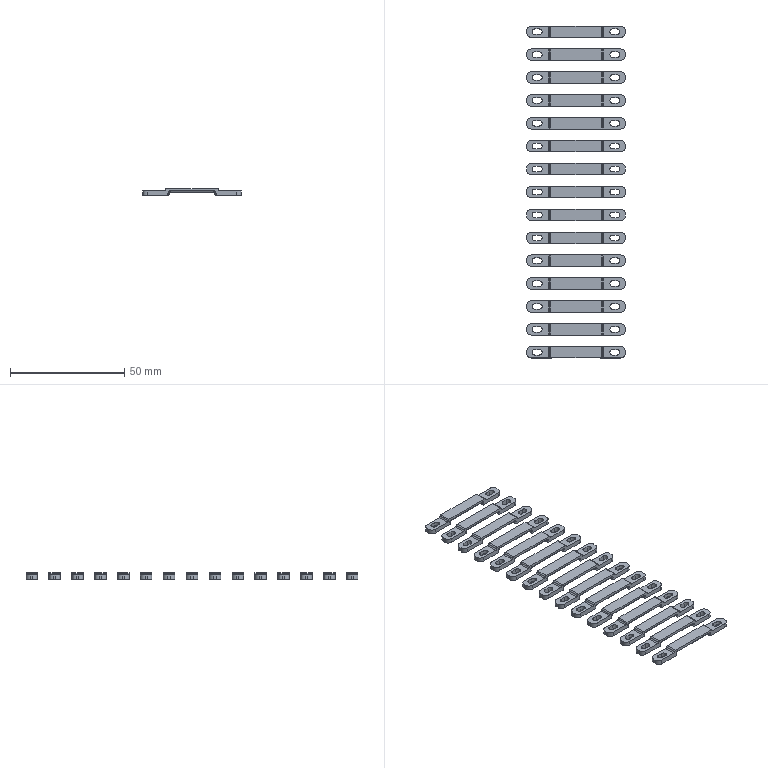NC program | NX | posted with a generic post | part box 43 x 145 x 3 mm
Lines 1 to 18 of 17881:
N10 G17 G21 G94 G90
(FLOOR_WALL , TOOL : D80)
N12 T19 M6
N14 G54
N16 G17 G0 G90 X117.5 Y0. S6500 M3
N18 G43 Z30. H19
N20 Z3.
N22 G94 G1 Z0. F1500.
N24 X114.5
N26 X-114.5
N28 X-117.5
N30 Z3.
N32 G0 Z30.
N34 M5